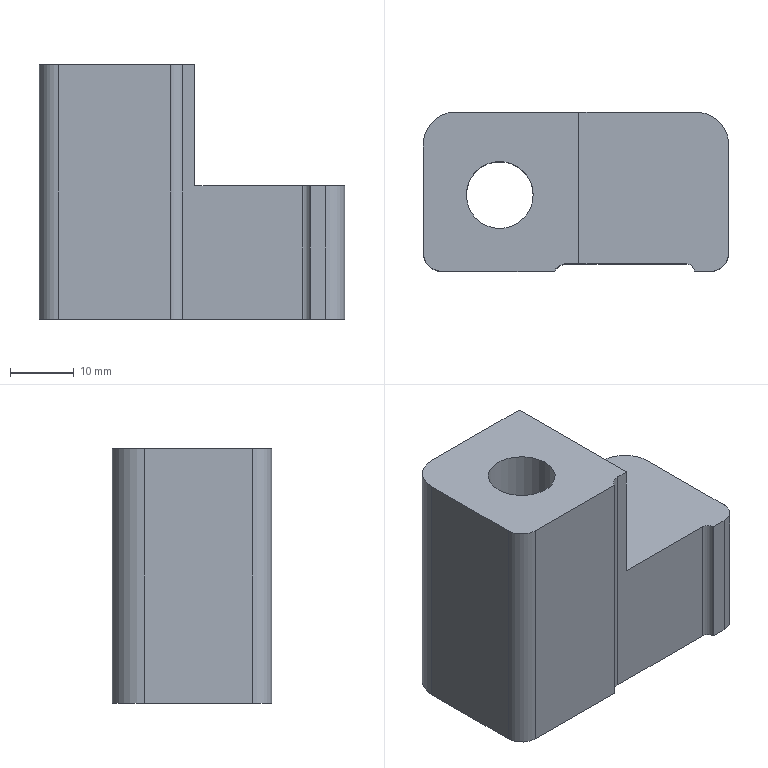Part | NX | features PS-12 2 | 1 solid | 19 faces | box 47.924 x 25 x 40 mm | volume 30062 mm3 | plane 11 | cylinder 8 | commonest cylinder face diameters 6 x2 10 x2 2.4 x1 4.4 x1 10.5 x1 18 x1
STEP:
#1=CARTESIAN_POINT('',(2543.009,-778.047,900.716));
#2=VERTEX_POINT('',#1);
#3=CARTESIAN_POINT('',(2543.009,-778.047,881.716));
#4=VERTEX_POINT('',#3);
#5=CARTESIAN_POINT('',(2543.009,-778.047,853.217));
#6=DIRECTION('',(0.,0.,1.));
#7=VECTOR('',#6,1000.);
#8=LINE('',#5,#7);
#9=EDGE_CURVE('',#2,#4,#8,.F.);
#10=ORIENTED_EDGE('',*,*,#9,.T.);
#11=CARTESIAN_POINT('',(2561.509,-778.047,881.716));
#12=VERTEX_POINT('',#11);
#13=CARTESIAN_POINT('',(2524.047,-778.047,881.716));
#14=DIRECTION('',(-1.,0.,0.));
#15=VECTOR('',#14,1000.);
#16=LINE('',#13,#15);
#17=EDGE_CURVE('',#12,#4,#16,.T.);
#18=ORIENTED_EDGE('',*,*,#17,.F.);
#19=CARTESIAN_POINT('',(2561.509,-778.047,860.716));
#20=VERTEX_POINT('',#19);
#21=CARTESIAN_POINT('',(2561.509,-778.047,853.217));
#22=DIRECTION('',(0.,0.,1.));
#23=VECTOR('',#22,1000.);
#24=LINE('',#21,#23);
#25=EDGE_CURVE('',#12,#20,#24,.F.);
#26=ORIENTED_EDGE('',*,*,#25,.T.);
#27=CARTESIAN_POINT('',(2523.585,-778.047,860.716));
#28=VERTEX_POINT('',#27);
#29=CARTESIAN_POINT('',(2524.047,-778.047,860.716));
#30=DIRECTION('',(-1.,0.,0.));
#31=VECTOR('',#30,1000.);
#32=LINE('',#29,#31);
#33=EDGE_CURVE('',#20,#28,#32,.T.);
#34=ORIENTED_EDGE('',*,*,#33,.T.);
#35=CARTESIAN_POINT('',(2523.585,-778.047,900.716));
#36=VERTEX_POINT('',#35);
#37=CARTESIAN_POINT('',(2523.585,-778.047,853.217));
#38=DIRECTION('',(0.,0.,1.));
#39=VECTOR('',#38,1000.);
#40=LINE('',#37,#39);
#41=EDGE_CURVE('',#28,#36,#40,.T.);
#42=ORIENTED_EDGE('',*,*,#41,.T.);
#43=CARTESIAN_POINT('',(2585.094,-778.047,900.716));
#44=DIRECTION('',(-1.,0.,0.));
#45=VECTOR('',#44,1000.);
#46=LINE('',#43,#45);
#47=EDGE_CURVE('',#2,#36,#46,.T.);
#48=ORIENTED_EDGE('',*,*,#47,.F.);
#49=EDGE_LOOP('',(#10,#18,#26,#34,#42,#48));
#50=FACE_BOUND('',#49,.T.);
#51=CARTESIAN_POINT('',(2524.047,-778.047,853.217));
#52=DIRECTION('',(0.,1.,0.));
#53=DIRECTION('',(0.,0.,1.));
#54=AXIS2_PLACEMENT_3D('',#51,#52,#53);
#55=PLANE('',#54);
#56=ADVANCED_FACE('',(#50),#55,.T.);
#57=CARTESIAN_POINT('',(2518.585,-783.047,900.716));
#58=VERTEX_POINT('',#57);
#59=CARTESIAN_POINT('',(2518.585,-783.047,860.716));
#60=VERTEX_POINT('',#59);
#61=CARTESIAN_POINT('',(2518.585,-783.047,875.716));
#62=DIRECTION('',(0.,0.,1.));
#63=VECTOR('',#62,1000.);
#64=LINE('',#61,#63);
#65=EDGE_CURVE('',#58,#60,#64,.F.);
#66=ORIENTED_EDGE('',*,*,#65,.T.);
#67=CARTESIAN_POINT('',(2518.585,-800.047,860.716));
#68=VERTEX_POINT('',#67);
#69=CARTESIAN_POINT('',(2518.585,-791.547,860.716));
#70=DIRECTION('',(0.,-1.,0.));
#71=VECTOR('',#70,1000.);
#72=LINE('',#69,#71);
#73=EDGE_CURVE('',#60,#68,#72,.T.);
#74=ORIENTED_EDGE('',*,*,#73,.T.);
#75=CARTESIAN_POINT('',(2518.585,-800.047,900.716));
#76=VERTEX_POINT('',#75);
#77=CARTESIAN_POINT('',(2518.585,-800.047,890.716));
#78=DIRECTION('',(0.,0.,1.));
#79=VECTOR('',#78,1000.);
#80=LINE('',#77,#79);
#81=EDGE_CURVE('',#68,#76,#80,.T.);
#82=ORIENTED_EDGE('',*,*,#81,.T.);
#83=CARTESIAN_POINT('',(2518.585,-859.122,900.716));
#84=DIRECTION('',(0.,-1.,0.));
#85=VECTOR('',#84,1000.);
#86=LINE('',#83,#85);
#87=EDGE_CURVE('',#58,#76,#86,.T.);
#88=ORIENTED_EDGE('',*,*,#87,.F.);
#89=EDGE_LOOP('',(#66,#74,#82,#88));
#90=FACE_BOUND('',#89,.T.);
#91=CARTESIAN_POINT('',(2518.585,-791.547,875.716));
#92=DIRECTION('',(-1.,0.,0.));
#93=DIRECTION('',(0.,0.,1.));
#94=AXIS2_PLACEMENT_3D('',#91,#92,#93);
#95=PLANE('',#94);
#96=ADVANCED_FACE('',(#90),#95,.T.);
#97=ORIENTED_EDGE('',*,*,#41,.F.);
#98=CARTESIAN_POINT('',(2523.585,-783.047,860.716));
#99=DIRECTION('',(0.,0.,-1.));
#100=DIRECTION('',(-1.,0.,0.));
#101=AXIS2_PLACEMENT_3D('',#98,#99,#100);
#102=CIRCLE('',#101,5.);
#103=EDGE_CURVE('',#60,#28,#102,.T.);
#104=ORIENTED_EDGE('',*,*,#103,.F.);
#105=ORIENTED_EDGE('',*,*,#65,.F.);
#106=CARTESIAN_POINT('',(2523.585,-783.047,900.716));
#107=DIRECTION('',(0.,0.,1.));
#108=DIRECTION('',(1.,0.,0.));
#109=AXIS2_PLACEMENT_3D('',#106,#107,#108);
#110=CIRCLE('',#109,5.);
#111=EDGE_CURVE('',#36,#58,#110,.T.);
#112=ORIENTED_EDGE('',*,*,#111,.F.);
#113=EDGE_LOOP('',(#97,#104,#105,#112));
#114=FACE_BOUND('',#113,.T.);
#115=CARTESIAN_POINT('',(2523.585,-783.047,853.217));
#116=DIRECTION('',(0.,0.,1.));
#117=DIRECTION('',(1.,0.,0.));
#118=AXIS2_PLACEMENT_3D('',#115,#116,#117);
#119=CYLINDRICAL_SURFACE('',#118,5.);
#120=ADVANCED_FACE('',(#114),#119,.T.);
#121=CARTESIAN_POINT('',(2539.585,-791.047,873.716));
#122=VERTEX_POINT('',#121);
#123=CARTESIAN_POINT('',(2530.585,-791.047,873.716));
#124=DIRECTION('',(0.,0.,-1.));
#125=DIRECTION('',(1.,0.,0.));
#126=AXIS2_PLACEMENT_3D('',#123,#124,#125);
#127=CIRCLE('',#126,9.);
#128=EDGE_CURVE('',#122,#122,#127,.F.);
#129=ORIENTED_EDGE('',*,*,#128,.T.);
#130=EDGE_LOOP('',(#129));
#131=FACE_BOUND('',#130,.T.);
#132=CARTESIAN_POINT('',(2521.585,-791.047,860.716));
#133=VERTEX_POINT('',#132);
#134=CARTESIAN_POINT('',(2530.585,-791.047,860.716));
#135=DIRECTION('',(0.,0.,-1.));
#136=DIRECTION('',(-1.,0.,0.));
#137=AXIS2_PLACEMENT_3D('',#134,#135,#136);
#138=CIRCLE('',#137,9.);
#139=EDGE_CURVE('',#133,#133,#138,.T.);
#140=ORIENTED_EDGE('',*,*,#139,.T.);
#141=EDGE_LOOP('',(#140));
#142=FACE_BOUND('',#141,.T.);
#143=CARTESIAN_POINT('',(2530.585,-791.047,873.716));
#144=DIRECTION('',(0.,0.,-1.));
#145=DIRECTION('',(-1.,0.,0.));
#146=AXIS2_PLACEMENT_3D('',#143,#144,#145);
#147=CYLINDRICAL_SURFACE('',#146,9.);
#148=ADVANCED_FACE('',(#131,#142),#147,.F.);
#149=CARTESIAN_POINT('',(2541.097,-801.847,860.716));
#150=VERTEX_POINT('',#149);
#151=CARTESIAN_POINT('',(2541.097,-801.847,900.716));
#152=VERTEX_POINT('',#151);
#153=CARTESIAN_POINT('',(2541.097,-801.847,889.83));
#154=DIRECTION('',(0.,0.,-1.));
#155=VECTOR('',#154,1000.);
#156=LINE('',#153,#155);
#157=EDGE_CURVE('',#150,#152,#156,.F.);
#158=ORIENTED_EDGE('',*,*,#157,.F.);
#159=CARTESIAN_POINT('',(2559.923,-801.847,860.716));
#160=VERTEX_POINT('',#159);
#161=CARTESIAN_POINT('',(2585.094,-801.847,860.716));
#162=DIRECTION('',(1.,0.,0.));
#163=VECTOR('',#162,1000.);
#164=LINE('',#161,#163);
#165=EDGE_CURVE('',#150,#160,#164,.T.);
#166=ORIENTED_EDGE('',*,*,#165,.T.);
#167=CARTESIAN_POINT('',(2559.923,-801.847,881.716));
#168=VERTEX_POINT('',#167);
#169=CARTESIAN_POINT('',(2559.923,-801.847,940.716));
#170=DIRECTION('',(0.,0.,1.));
#171=VECTOR('',#170,1000.);
#172=LINE('',#169,#171);
#173=EDGE_CURVE('',#160,#168,#172,.T.);
#174=ORIENTED_EDGE('',*,*,#173,.T.);
#175=CARTESIAN_POINT('',(2543.009,-801.847,881.716));
#176=VERTEX_POINT('',#175);
#177=CARTESIAN_POINT('',(2542.547,-801.847,881.716));
#178=DIRECTION('',(1.,0.,0.));
#179=VECTOR('',#178,1000.);
#180=LINE('',#177,#179);
#181=EDGE_CURVE('',#176,#168,#180,.T.);
#182=ORIENTED_EDGE('',*,*,#181,.F.);
#183=CARTESIAN_POINT('',(2543.009,-801.847,900.716));
#184=VERTEX_POINT('',#183);
#185=CARTESIAN_POINT('',(2543.009,-801.847,940.716));
#186=DIRECTION('',(0.,0.,1.));
#187=VECTOR('',#186,1000.);
#188=LINE('',#185,#187);
#189=EDGE_CURVE('',#176,#184,#188,.T.);
#190=ORIENTED_EDGE('',*,*,#189,.T.);
#191=CARTESIAN_POINT('',(2585.094,-801.847,900.716));
#192=DIRECTION('',(-1.,0.,0.));
#193=VECTOR('',#192,1000.);
#194=LINE('',#191,#193);
#195=EDGE_CURVE('',#184,#152,#194,.T.);
#196=ORIENTED_EDGE('',*,*,#195,.T.);
#197=EDGE_LOOP('',(#158,#166,#174,#182,#190,#196));
#198=FACE_BOUND('',#197,.T.);
#199=CARTESIAN_POINT('',(2656.665,-801.847,940.716));
#200=DIRECTION('',(0.,1.,0.));
#201=DIRECTION('',(0.,0.,1.));
#202=AXIS2_PLACEMENT_3D('',#199,#200,#201);
#203=PLANE('',#202);
#204=ADVANCED_FACE('',(#198),#203,.F.);
#205=CARTESIAN_POINT('',(2539.137,-803.047,900.716));
#206=VERTEX_POINT('',#205);
#207=CARTESIAN_POINT('',(2539.137,-803.047,860.716));
#208=VERTEX_POINT('',#207);
#209=CARTESIAN_POINT('',(2539.137,-803.047,890.716));
#210=DIRECTION('',(0.,0.,-1.));
#211=VECTOR('',#210,1000.);
#212=LINE('',#209,#211);
#213=EDGE_CURVE('',#206,#208,#212,.T.);
#214=ORIENTED_EDGE('',*,*,#213,.T.);
#215=CARTESIAN_POINT('',(2541.097,-804.047,860.716));
#216=DIRECTION('',(0.,0.,-1.));
#217=DIRECTION('',(-1.,0.,0.));
#218=AXIS2_PLACEMENT_3D('',#215,#216,#217);
#219=CIRCLE('',#218,2.2);
#220=EDGE_CURVE('',#208,#150,#219,.T.);
#221=ORIENTED_EDGE('',*,*,#220,.T.);
#222=ORIENTED_EDGE('',*,*,#157,.T.);
#223=CARTESIAN_POINT('',(2541.097,-804.047,900.716));
#224=DIRECTION('',(0.,0.,1.));
#225=DIRECTION('',(1.,0.,0.));
#226=AXIS2_PLACEMENT_3D('',#223,#224,#225);
#227=CIRCLE('',#226,2.2);
#228=EDGE_CURVE('',#152,#206,#227,.T.);
#229=ORIENTED_EDGE('',*,*,#228,.T.);
#230=EDGE_LOOP('',(#214,#221,#222,#229));
#231=FACE_BOUND('',#230,.T.);
#232=CARTESIAN_POINT('',(2541.097,-804.047,889.83));
#233=DIRECTION('',(0.,0.,-1.));
#234=DIRECTION('',(-1.,0.,0.));
#235=AXIS2_PLACEMENT_3D('',#232,#233,#234);
#236=CYLINDRICAL_SURFACE('',#235,2.2);
#237=ADVANCED_FACE('',(#231),#236,.F.);
#238=CARTESIAN_POINT('',(2521.585,-803.047,900.716));
#239=VERTEX_POINT('',#238);
#240=CARTESIAN_POINT('',(2521.585,-803.047,860.716));
#241=VERTEX_POINT('',#240);
#242=CARTESIAN_POINT('',(2521.585,-803.047,860.716));
#243=DIRECTION('',(0.,0.,1.));
#244=VECTOR('',#243,1000.);
#245=LINE('',#242,#244);
#246=EDGE_CURVE('',#239,#241,#245,.F.);
#247=ORIENTED_EDGE('',*,*,#246,.T.);
#248=CARTESIAN_POINT('',(2585.094,-803.047,860.716));
#249=DIRECTION('',(1.,0.,0.));
#250=VECTOR('',#249,1000.);
#251=LINE('',#248,#250);
#252=EDGE_CURVE('',#241,#208,#251,.T.);
#253=ORIENTED_EDGE('',*,*,#252,.T.);
#254=ORIENTED_EDGE('',*,*,#213,.F.);
#255=CARTESIAN_POINT('',(2550.509,-803.047,900.716));
#256=DIRECTION('',(1.,0.,0.));
#257=VECTOR('',#256,1000.);
#258=LINE('',#255,#257);
#259=EDGE_CURVE('',#239,#206,#258,.T.);
#260=ORIENTED_EDGE('',*,*,#259,.F.);
#261=EDGE_LOOP('',(#247,#253,#254,#260));
#262=FACE_BOUND('',#261,.T.);
#263=CARTESIAN_POINT('',(2550.509,-803.047,895.794));
#264=DIRECTION('',(0.,1.,0.));
#265=DIRECTION('',(0.,0.,1.));
#266=AXIS2_PLACEMENT_3D('',#263,#264,#265);
#267=PLANE('',#266);
#268=ADVANCED_FACE('',(#262),#267,.F.);
#269=ORIENTED_EDGE('',*,*,#81,.F.);
#270=CARTESIAN_POINT('',(2521.585,-800.047,860.716));
#271=DIRECTION('',(0.,0.,-1.));
#272=DIRECTION('',(-1.,0.,0.));
#273=AXIS2_PLACEMENT_3D('',#270,#271,#272);
#274=CIRCLE('',#273,3.);
#275=EDGE_CURVE('',#241,#68,#274,.T.);
#276=ORIENTED_EDGE('',*,*,#275,.F.);
#277=ORIENTED_EDGE('',*,*,#246,.F.);
#278=CARTESIAN_POINT('',(2521.585,-800.047,900.716));
#279=DIRECTION('',(0.,0.,1.));
#280=DIRECTION('',(1.,0.,0.));
#281=AXIS2_PLACEMENT_3D('',#278,#279,#280);
#282=CIRCLE('',#281,3.);
#283=EDGE_CURVE('',#76,#239,#282,.T.);
#284=ORIENTED_EDGE('',*,*,#283,.F.);
#285=EDGE_LOOP('',(#269,#276,#277,#284));
#286=FACE_BOUND('',#285,.T.);
#287=CARTESIAN_POINT('',(2521.585,-800.047,875.716));
#288=DIRECTION('',(0.,0.,-1.));
#289=DIRECTION('',(-1.,0.,0.));
#290=AXIS2_PLACEMENT_3D('',#287,#288,#289);
#291=CYLINDRICAL_SURFACE('',#290,3.);
#292=ADVANCED_FACE('',(#286),#291,.T.);
#293=CARTESIAN_POINT('',(2543.009,-859.122,900.716));
#294=DIRECTION('',(0.,-1.,0.));
#295=VECTOR('',#294,1000.);
#296=LINE('',#293,#295);
#297=EDGE_CURVE('',#184,#2,#296,.F.);
#298=ORIENTED_EDGE('',*,*,#297,.T.);
#299=ORIENTED_EDGE('',*,*,#47,.T.);
#300=ORIENTED_EDGE('',*,*,#111,.T.);
#301=ORIENTED_EDGE('',*,*,#87,.T.);
#302=ORIENTED_EDGE('',*,*,#283,.T.);
#303=ORIENTED_EDGE('',*,*,#259,.T.);
#304=ORIENTED_EDGE('',*,*,#228,.F.);
#305=ORIENTED_EDGE('',*,*,#195,.F.);
#306=EDGE_LOOP('',(#298,#299,#300,#301,#302,#303,#304,#305));
#307=FACE_BOUND('',#306,.T.);
#308=CARTESIAN_POINT('',(2535.835,-791.047,900.716));
#309=VERTEX_POINT('',#308);
#310=CARTESIAN_POINT('',(2530.585,-791.047,900.716));
#311=DIRECTION('',(0.,0.,1.));
#312=DIRECTION('',(1.,0.,0.));
#313=AXIS2_PLACEMENT_3D('',#310,#311,#312);
#314=CIRCLE('',#313,5.25);
#315=EDGE_CURVE('',#309,#309,#314,.T.);
#316=ORIENTED_EDGE('',*,*,#315,.F.);
#317=EDGE_LOOP('',(#316));
#318=FACE_BOUND('',#317,.T.);
#319=CARTESIAN_POINT('',(2585.094,-859.122,900.716));
#320=DIRECTION('',(0.,0.,1.));
#321=DIRECTION('',(1.,0.,0.));
#322=AXIS2_PLACEMENT_3D('',#319,#320,#321);
#323=PLANE('',#322);
#324=ADVANCED_FACE('',(#307,#318),#323,.T.);
#325=ORIENTED_EDGE('',*,*,#315,.T.);
#326=EDGE_LOOP('',(#325));
#327=FACE_BOUND('',#326,.T.);
#328=CARTESIAN_POINT('',(2525.335,-791.047,873.716));
#329=VERTEX_POINT('',#328);
#330=CARTESIAN_POINT('',(2530.585,-791.047,873.716));
#331=DIRECTION('',(0.,0.,-1.));
#332=DIRECTION('',(-1.,0.,0.));
#333=AXIS2_PLACEMENT_3D('',#330,#331,#332);
#334=CIRCLE('',#333,5.25);
#335=EDGE_CURVE('',#329,#329,#334,.T.);
#336=ORIENTED_EDGE('',*,*,#335,.T.);
#337=EDGE_LOOP('',(#336));
#338=FACE_BOUND('',#337,.T.);
#339=CARTESIAN_POINT('',(2530.585,-791.047,891.716));
#340=DIRECTION('',(0.,0.,-1.));
#341=DIRECTION('',(-1.,0.,0.));
#342=AXIS2_PLACEMENT_3D('',#339,#340,#341);
#343=CYLINDRICAL_SURFACE('',#342,5.25);
#344=ADVANCED_FACE('',(#327,#338),#343,.F.);
#345=ORIENTED_EDGE('',*,*,#335,.F.);
#346=EDGE_LOOP('',(#345));
#347=FACE_BOUND('',#346,.T.);
#348=ORIENTED_EDGE('',*,*,#128,.F.);
#349=EDGE_LOOP('',(#348));
#350=FACE_BOUND('',#349,.T.);
#351=CARTESIAN_POINT('',(2530.585,-791.047,873.716));
#352=DIRECTION('',(0.,0.,-1.));
#353=DIRECTION('',(-1.,0.,0.));
#354=AXIS2_PLACEMENT_3D('',#351,#352,#353);
#355=PLANE('',#354);
#356=ADVANCED_FACE('',(#347,#350),#355,.T.);
#357=ORIENTED_EDGE('',*,*,#297,.F.);
#358=ORIENTED_EDGE('',*,*,#189,.F.);
#359=CARTESIAN_POINT('',(2543.009,-792.297,881.716));
#360=DIRECTION('',(0.,-1.,0.));
#361=VECTOR('',#360,1000.);
#362=LINE('',#359,#361);
#363=EDGE_CURVE('',#4,#176,#362,.T.);
#364=ORIENTED_EDGE('',*,*,#363,.F.);
#365=ORIENTED_EDGE('',*,*,#9,.F.);
#366=EDGE_LOOP('',(#357,#358,#364,#365));
#367=FACE_BOUND('',#366,.T.);
#368=CARTESIAN_POINT('',(2543.009,-792.297,911.056));
#369=DIRECTION('',(-1.,0.,0.));
#370=DIRECTION('',(0.,0.,1.));
#371=AXIS2_PLACEMENT_3D('',#368,#369,#370);
#372=PLANE('',#371);
#373=ADVANCED_FACE('',(#367),#372,.F.);
#374=ORIENTED_EDGE('',*,*,#17,.T.);
#375=ORIENTED_EDGE('',*,*,#363,.T.);
#376=ORIENTED_EDGE('',*,*,#181,.T.);
#377=CARTESIAN_POINT('',(2561.123,-803.047,881.716));
#378=VERTEX_POINT('',#377);
#379=CARTESIAN_POINT('',(2559.923,-803.047,881.716));
#380=DIRECTION('',(0.,0.,-1.));
#381=DIRECTION('',(-1.,0.,0.));
#382=AXIS2_PLACEMENT_3D('',#379,#380,#381);
#383=CIRCLE('',#382,1.2);
#384=EDGE_CURVE('',#378,#168,#383,.F.);
#385=ORIENTED_EDGE('',*,*,#384,.F.);
#386=CARTESIAN_POINT('',(2563.509,-803.047,881.716));
#387=VERTEX_POINT('',#386);
#388=CARTESIAN_POINT('',(2550.509,-803.047,881.716));
#389=DIRECTION('',(-1.,0.,0.));
#390=VECTOR('',#389,1000.);
#391=LINE('',#388,#390);
#392=EDGE_CURVE('',#387,#378,#391,.T.);
#393=ORIENTED_EDGE('',*,*,#392,.F.);
#394=CARTESIAN_POINT('',(2566.509,-800.047,881.716));
#395=VERTEX_POINT('',#394);
#396=CARTESIAN_POINT('',(2563.509,-800.047,881.716));
#397=DIRECTION('',(0.,0.,-1.));
#398=DIRECTION('',(-1.,0.,0.));
#399=AXIS2_PLACEMENT_3D('',#396,#397,#398);
#400=CIRCLE('',#399,3.);
#401=EDGE_CURVE('',#387,#395,#400,.F.);
#402=ORIENTED_EDGE('',*,*,#401,.T.);
#403=CARTESIAN_POINT('',(2566.509,-783.047,881.716));
#404=VERTEX_POINT('',#403);
#405=CARTESIAN_POINT('',(2566.509,-810.085,881.716));
#406=DIRECTION('',(0.,1.,0.));
#407=VECTOR('',#406,1000.);
#408=LINE('',#405,#407);
#409=EDGE_CURVE('',#395,#404,#408,.T.);
#410=ORIENTED_EDGE('',*,*,#409,.T.);
#411=CARTESIAN_POINT('',(2561.509,-783.047,881.716));
#412=DIRECTION('',(0.,0.,-1.));
#413=DIRECTION('',(-1.,0.,0.));
#414=AXIS2_PLACEMENT_3D('',#411,#412,#413);
#415=CIRCLE('',#414,5.);
#416=EDGE_CURVE('',#404,#12,#415,.F.);
#417=ORIENTED_EDGE('',*,*,#416,.T.);
#418=EDGE_LOOP('',(#374,#375,#376,#385,#393,#402,#410,#417));
#419=FACE_BOUND('',#418,.T.);
#420=CARTESIAN_POINT('',(2542.547,-790.547,881.716));
#421=DIRECTION('',(0.,0.,-1.));
#422=DIRECTION('',(-1.,0.,0.));
#423=AXIS2_PLACEMENT_3D('',#420,#421,#422);
#424=PLANE('',#423);
#425=ADVANCED_FACE('',(#419),#424,.F.);
#426=ORIENTED_EDGE('',*,*,#252,.F.);
#427=ORIENTED_EDGE('',*,*,#275,.T.);
#428=ORIENTED_EDGE('',*,*,#73,.F.);
#429=ORIENTED_EDGE('',*,*,#103,.T.);
#430=ORIENTED_EDGE('',*,*,#33,.F.);
#431=CARTESIAN_POINT('',(2566.509,-783.047,860.716));
#432=VERTEX_POINT('',#431);
#433=CARTESIAN_POINT('',(2561.509,-783.047,860.716));
#434=DIRECTION('',(0.,0.,-1.));
#435=DIRECTION('',(-1.,0.,0.));
#436=AXIS2_PLACEMENT_3D('',#433,#434,#435);
#437=CIRCLE('',#436,5.);
#438=EDGE_CURVE('',#20,#432,#437,.T.);
#439=ORIENTED_EDGE('',*,*,#438,.T.);
#440=CARTESIAN_POINT('',(2566.509,-800.047,860.716));
#441=VERTEX_POINT('',#440);
#442=CARTESIAN_POINT('',(2566.509,-859.122,860.716));
#443=DIRECTION('',(0.,-1.,0.));
#444=VECTOR('',#443,1000.);
#445=LINE('',#442,#444);
#446=EDGE_CURVE('',#432,#441,#445,.T.);
#447=ORIENTED_EDGE('',*,*,#446,.T.);
#448=CARTESIAN_POINT('',(2563.509,-803.047,860.716));
#449=VERTEX_POINT('',#448);
#450=CARTESIAN_POINT('',(2563.509,-800.047,860.716));
#451=DIRECTION('',(0.,0.,-1.));
#452=DIRECTION('',(-1.,0.,0.));
#453=AXIS2_PLACEMENT_3D('',#450,#451,#452);
#454=CIRCLE('',#453,3.);
#455=EDGE_CURVE('',#441,#449,#454,.T.);
#456=ORIENTED_EDGE('',*,*,#455,.T.);
#457=CARTESIAN_POINT('',(2561.123,-803.047,860.716));
#458=VERTEX_POINT('',#457);
#459=CARTESIAN_POINT('',(2585.094,-803.047,860.716));
#460=DIRECTION('',(1.,0.,0.));
#461=VECTOR('',#460,1000.);
#462=LINE('',#459,#461);
#463=EDGE_CURVE('',#458,#449,#462,.T.);
#464=ORIENTED_EDGE('',*,*,#463,.F.);
#465=CARTESIAN_POINT('',(2559.923,-803.047,860.716));
#466=DIRECTION('',(0.,0.,-1.));
#467=DIRECTION('',(-1.,0.,0.));
#468=AXIS2_PLACEMENT_3D('',#465,#466,#467);
#469=CIRCLE('',#468,1.2);
#470=EDGE_CURVE('',#458,#160,#469,.F.);
#471=ORIENTED_EDGE('',*,*,#470,.T.);
#472=ORIENTED_EDGE('',*,*,#165,.F.);
#473=ORIENTED_EDGE('',*,*,#220,.F.);
#474=EDGE_LOOP('',(#426,#427,#428,#429,#430,#439,#447,#456,#464,#471,#472,#473));
#475=FACE_BOUND('',#474,.T.);
#476=ORIENTED_EDGE('',*,*,#139,.F.);
#477=EDGE_LOOP('',(#476));
#478=FACE_BOUND('',#477,.T.);
#479=CARTESIAN_POINT('',(2585.094,-859.122,860.716));
#480=DIRECTION('',(0.,0.,-1.));
#481=DIRECTION('',(-1.,0.,0.));
#482=AXIS2_PLACEMENT_3D('',#479,#480,#481);
#483=PLANE('',#482);
#484=ADVANCED_FACE('',(#475,#478),#483,.T.);
#485=ORIENTED_EDGE('',*,*,#401,.F.);
#486=CARTESIAN_POINT('',(2563.509,-803.047,890.716));
#487=DIRECTION('',(0.,0.,1.));
#488=VECTOR('',#487,1000.);
#489=LINE('',#486,#488);
#490=EDGE_CURVE('',#449,#387,#489,.T.);
#491=ORIENTED_EDGE('',*,*,#490,.F.);
#492=ORIENTED_EDGE('',*,*,#455,.F.);
#493=CARTESIAN_POINT('',(2566.509,-800.047,860.716));
#494=DIRECTION('',(0.,0.,1.));
#495=VECTOR('',#494,1000.);
#496=LINE('',#493,#495);
#497=EDGE_CURVE('',#395,#441,#496,.F.);
#498=ORIENTED_EDGE('',*,*,#497,.F.);
#499=EDGE_LOOP('',(#485,#491,#492,#498));
#500=FACE_BOUND('',#499,.T.);
#501=CARTESIAN_POINT('',(2563.509,-800.047,895.794));
#502=DIRECTION('',(0.,0.,-1.));
#503=DIRECTION('',(-1.,0.,0.));
#504=AXIS2_PLACEMENT_3D('',#501,#502,#503);
#505=CYLINDRICAL_SURFACE('',#504,3.);
#506=ADVANCED_FACE('',(#500),#505,.T.);
#507=ORIENTED_EDGE('',*,*,#490,.T.);
#508=ORIENTED_EDGE('',*,*,#392,.T.);
#509=CARTESIAN_POINT('',(2561.123,-803.047,940.716));
#510=DIRECTION('',(0.,0.,1.));
#511=VECTOR('',#510,1000.);
#512=LINE('',#509,#511);
#513=EDGE_CURVE('',#378,#458,#512,.F.);
#514=ORIENTED_EDGE('',*,*,#513,.T.);
#515=ORIENTED_EDGE('',*,*,#463,.T.);
#516=EDGE_LOOP('',(#507,#508,#514,#515));
#517=FACE_BOUND('',#516,.T.);
#518=CARTESIAN_POINT('',(2550.509,-803.047,895.794));
#519=DIRECTION('',(0.,1.,0.));
#520=DIRECTION('',(0.,0.,1.));
#521=AXIS2_PLACEMENT_3D('',#518,#519,#520);
#522=PLANE('',#521);
#523=ADVANCED_FACE('',(#517),#522,.F.);
#524=ORIENTED_EDGE('',*,*,#384,.T.);
#525=ORIENTED_EDGE('',*,*,#173,.F.);
#526=ORIENTED_EDGE('',*,*,#470,.F.);
#527=ORIENTED_EDGE('',*,*,#513,.F.);
#528=EDGE_LOOP('',(#524,#525,#526,#527));
#529=FACE_BOUND('',#528,.T.);
#530=CARTESIAN_POINT('',(2559.923,-803.047,940.716));
#531=DIRECTION('',(0.,0.,1.));
#532=DIRECTION('',(1.,0.,0.));
#533=AXIS2_PLACEMENT_3D('',#530,#531,#532);
#534=CYLINDRICAL_SURFACE('',#533,1.2);
#535=ADVANCED_FACE('',(#529),#534,.F.);
#536=ORIENTED_EDGE('',*,*,#416,.F.);
#537=CARTESIAN_POINT('',(2566.509,-783.047,853.217));
#538=DIRECTION('',(0.,0.,1.));
#539=VECTOR('',#538,1000.);
#540=LINE('',#537,#539);
#541=EDGE_CURVE('',#432,#404,#540,.T.);
#542=ORIENTED_EDGE('',*,*,#541,.F.);
#543=ORIENTED_EDGE('',*,*,#438,.F.);
#544=ORIENTED_EDGE('',*,*,#25,.F.);
#545=EDGE_LOOP('',(#536,#542,#543,#544));
#546=FACE_BOUND('',#545,.T.);
#547=CARTESIAN_POINT('',(2561.509,-783.047,853.217));
#548=DIRECTION('',(0.,0.,1.));
#549=DIRECTION('',(1.,0.,0.));
#550=AXIS2_PLACEMENT_3D('',#547,#548,#549);
#551=CYLINDRICAL_SURFACE('',#550,5.);
#552=ADVANCED_FACE('',(#546),#551,.T.);
#553=ORIENTED_EDGE('',*,*,#409,.F.);
#554=ORIENTED_EDGE('',*,*,#497,.T.);
#555=ORIENTED_EDGE('',*,*,#446,.F.);
#556=ORIENTED_EDGE('',*,*,#541,.T.);
#557=EDGE_LOOP('',(#553,#554,#555,#556));
#558=FACE_BOUND('',#557,.T.);
#559=CARTESIAN_POINT('',(2566.509,-810.085,853.217));
#560=DIRECTION('',(1.,0.,0.));
#561=DIRECTION('',(0.,0.,-1.));
#562=AXIS2_PLACEMENT_3D('',#559,#560,#561);
#563=PLANE('',#562);
#564=ADVANCED_FACE('',(#558),#563,.T.);
#565=CLOSED_SHELL('',(#56,#96,#120,#148,#204,#237,#268,#292,#324,#344,#356,#373,#425,#484,#506,#523,#535,#552,#564));
#566=MANIFOLD_SOLID_BREP('',#565);
#567=(LENGTH_UNIT()NAMED_UNIT(*)SI_UNIT(.MILLI.,.METRE.));
#568=UNCERTAINTY_MEASURE_WITH_UNIT(LENGTH_MEASURE(0.00001),#567,'','');
#569=(NAMED_UNIT(*)PLANE_ANGLE_UNIT()SI_UNIT($,.RADIAN.));
#570=(NAMED_UNIT(*)SI_UNIT($,.STERADIAN.)SOLID_ANGLE_UNIT());
#571=(GEOMETRIC_REPRESENTATION_CONTEXT(3)GLOBAL_UNCERTAINTY_ASSIGNED_CONTEXT((#568))GLOBAL_UNIT_ASSIGNED_CONTEXT((#567,#569,#570))REPRESENTATION_CONTEXT('',''));
#572=ADVANCED_BREP_SHAPE_REPRESENTATION('',(#566),#571);